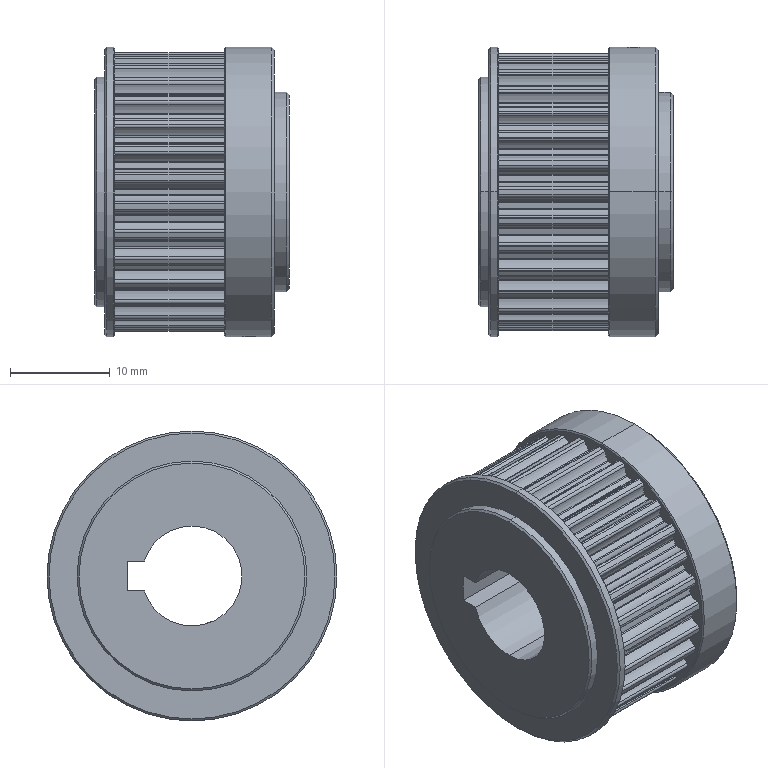Part | STEP file | 1 solid | 304 faces | box 19.5 x 29 x 29 mm | volume 9304 mm3 | cylinder 280 | cone 15 | plane 9 | commonest cylinder face diameters 0.56 x72 0.3 x68 3.95 x64 27.89 x31 25.67 x30 2.5 x4